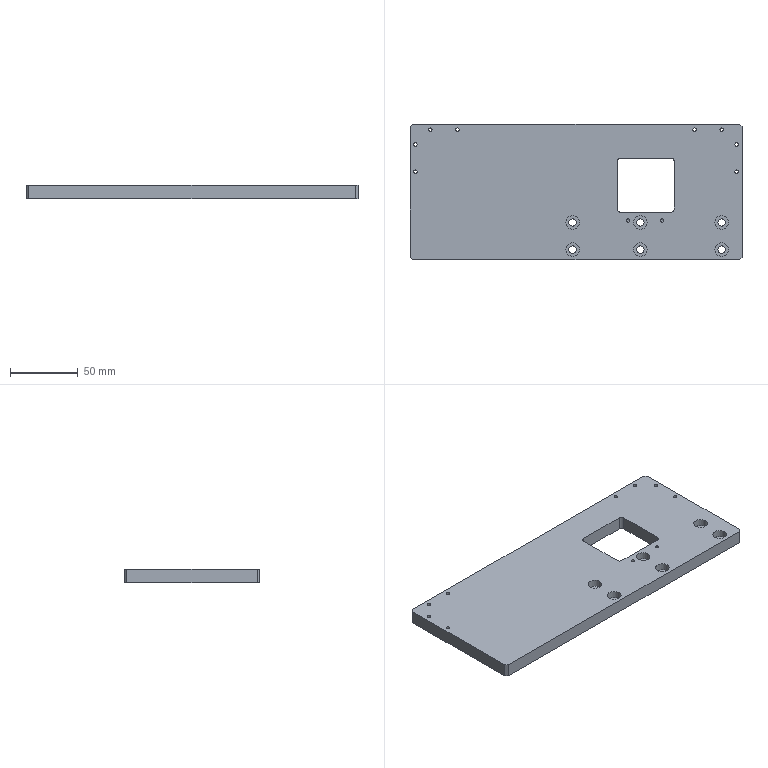Part | 1 solid | 48 faces | box 245 x 100 x 10 mm | volume 224502 mm3 | cylinder 26 | plane 20 | cone 2 | commonest cylinder face diameters 2.5 x10 5.5 x6 10 x6 4.871 x4
STEP:
#1=CARTESIAN_POINT('',(32.935,-15.,5.));
#2=VERTEX_POINT('',#1);
#3=CARTESIAN_POINT('',(70.065,-15.,5.));
#4=VERTEX_POINT('',#3);
#5=CARTESIAN_POINT('',(70.065,-15.,5.));
#6=DIRECTION('',(1.,0.,0.));
#7=VECTOR('',#6,1000.);
#8=LINE('',#5,#7);
#9=EDGE_CURVE('',#2,#4,#8,.T.);
#10=ORIENTED_EDGE('',*,*,#9,.T.);
#11=CARTESIAN_POINT('',(70.065,-15.,-5.));
#12=VERTEX_POINT('',#11);
#13=CARTESIAN_POINT('',(70.065,-15.,-5.));
#14=DIRECTION('',(0.,0.,1.));
#15=VECTOR('',#14,1000.);
#16=LINE('',#13,#15);
#17=EDGE_CURVE('',#12,#4,#16,.T.);
#18=ORIENTED_EDGE('',*,*,#17,.F.);
#19=CARTESIAN_POINT('',(32.935,-15.,-5.));
#20=VERTEX_POINT('',#19);
#21=CARTESIAN_POINT('',(70.065,-15.,-5.));
#22=DIRECTION('',(1.,0.,0.));
#23=VECTOR('',#22,1000.);
#24=LINE('',#21,#23);
#25=EDGE_CURVE('',#20,#12,#24,.T.);
#26=ORIENTED_EDGE('',*,*,#25,.F.);
#27=CARTESIAN_POINT('',(32.935,-15.,-5.));
#28=DIRECTION('',(0.,0.,1.));
#29=VECTOR('',#28,1000.);
#30=LINE('',#27,#29);
#31=EDGE_CURVE('',#20,#2,#30,.T.);
#32=ORIENTED_EDGE('',*,*,#31,.T.);
#33=EDGE_LOOP('',(#10,#18,#26,#32));
#34=FACE_BOUND('',#33,.T.);
#35=CARTESIAN_POINT('',(70.065,-15.,-5.));
#36=DIRECTION('',(0.,-1.,0.));
#37=DIRECTION('',(1.,0.,0.));
#38=AXIS2_PLACEMENT_3D('',#35,#36,#37);
#39=PLANE('',#38);
#40=ADVANCED_FACE('',(#34),#39,.F.);
#41=CARTESIAN_POINT('',(72.5,-12.565,5.));
#42=VERTEX_POINT('',#41);
#43=CARTESIAN_POINT('',(70.065,-12.565,5.));
#44=DIRECTION('',(0.,0.,1.));
#45=DIRECTION('',(1.,0.,0.));
#46=AXIS2_PLACEMENT_3D('',#43,#44,#45);
#47=CIRCLE('',#46,2.435);
#48=EDGE_CURVE('',#4,#42,#47,.T.);
#49=ORIENTED_EDGE('',*,*,#48,.T.);
#50=CARTESIAN_POINT('',(72.5,-12.565,-5.));
#51=VERTEX_POINT('',#50);
#52=CARTESIAN_POINT('',(72.5,-12.565,-5.));
#53=DIRECTION('',(0.,0.,1.));
#54=VECTOR('',#53,1000.);
#55=LINE('',#52,#54);
#56=EDGE_CURVE('',#51,#42,#55,.T.);
#57=ORIENTED_EDGE('',*,*,#56,.F.);
#58=CARTESIAN_POINT('',(70.065,-12.565,-5.));
#59=DIRECTION('',(0.,0.,1.));
#60=DIRECTION('',(1.,0.,0.));
#61=AXIS2_PLACEMENT_3D('',#58,#59,#60);
#62=CIRCLE('',#61,2.435);
#63=EDGE_CURVE('',#12,#51,#62,.T.);
#64=ORIENTED_EDGE('',*,*,#63,.F.);
#65=ORIENTED_EDGE('',*,*,#17,.T.);
#66=EDGE_LOOP('',(#49,#57,#64,#65));
#67=FACE_BOUND('',#66,.T.);
#68=CARTESIAN_POINT('',(70.065,-12.565,-5.));
#69=DIRECTION('',(0.,0.,1.));
#70=DIRECTION('',(1.,0.,0.));
#71=AXIS2_PLACEMENT_3D('',#68,#69,#70);
#72=CYLINDRICAL_SURFACE('',#71,2.435);
#73=ADVANCED_FACE('',(#67),#72,.F.);
#74=CARTESIAN_POINT('',(72.5,22.565,5.));
#75=VERTEX_POINT('',#74);
#76=CARTESIAN_POINT('',(72.5,-12.565,5.));
#77=DIRECTION('',(0.,1.,0.));
#78=VECTOR('',#77,1000.);
#79=LINE('',#76,#78);
#80=EDGE_CURVE('',#42,#75,#79,.T.);
#81=ORIENTED_EDGE('',*,*,#80,.T.);
#82=CARTESIAN_POINT('',(72.5,22.565,-5.));
#83=VERTEX_POINT('',#82);
#84=CARTESIAN_POINT('',(72.5,22.565,-5.));
#85=DIRECTION('',(0.,0.,1.));
#86=VECTOR('',#85,1000.);
#87=LINE('',#84,#86);
#88=EDGE_CURVE('',#83,#75,#87,.T.);
#89=ORIENTED_EDGE('',*,*,#88,.F.);
#90=CARTESIAN_POINT('',(72.5,-12.565,-5.));
#91=DIRECTION('',(0.,1.,0.));
#92=VECTOR('',#91,1000.);
#93=LINE('',#90,#92);
#94=EDGE_CURVE('',#51,#83,#93,.T.);
#95=ORIENTED_EDGE('',*,*,#94,.F.);
#96=ORIENTED_EDGE('',*,*,#56,.T.);
#97=EDGE_LOOP('',(#81,#89,#95,#96));
#98=FACE_BOUND('',#97,.T.);
#99=CARTESIAN_POINT('',(72.5,-12.565,-5.));
#100=DIRECTION('',(1.,0.,0.));
#101=DIRECTION('',(0.,0.,-1.));
#102=AXIS2_PLACEMENT_3D('',#99,#100,#101);
#103=PLANE('',#102);
#104=ADVANCED_FACE('',(#98),#103,.F.);
#105=CARTESIAN_POINT('',(70.065,25.,5.));
#106=VERTEX_POINT('',#105);
#107=CARTESIAN_POINT('',(70.065,22.565,5.));
#108=DIRECTION('',(0.,0.,1.));
#109=DIRECTION('',(1.,0.,0.));
#110=AXIS2_PLACEMENT_3D('',#107,#108,#109);
#111=CIRCLE('',#110,2.435);
#112=EDGE_CURVE('',#75,#106,#111,.T.);
#113=ORIENTED_EDGE('',*,*,#112,.T.);
#114=CARTESIAN_POINT('',(70.065,25.,-5.));
#115=VERTEX_POINT('',#114);
#116=CARTESIAN_POINT('',(70.065,25.,-5.));
#117=DIRECTION('',(0.,0.,1.));
#118=VECTOR('',#117,1000.);
#119=LINE('',#116,#118);
#120=EDGE_CURVE('',#115,#106,#119,.T.);
#121=ORIENTED_EDGE('',*,*,#120,.F.);
#122=CARTESIAN_POINT('',(70.065,22.565,-5.));
#123=DIRECTION('',(0.,0.,1.));
#124=DIRECTION('',(1.,0.,0.));
#125=AXIS2_PLACEMENT_3D('',#122,#123,#124);
#126=CIRCLE('',#125,2.435);
#127=EDGE_CURVE('',#83,#115,#126,.T.);
#128=ORIENTED_EDGE('',*,*,#127,.F.);
#129=ORIENTED_EDGE('',*,*,#88,.T.);
#130=EDGE_LOOP('',(#113,#121,#128,#129));
#131=FACE_BOUND('',#130,.T.);
#132=CARTESIAN_POINT('',(70.065,22.565,-5.));
#133=DIRECTION('',(0.,0.,1.));
#134=DIRECTION('',(1.,0.,0.));
#135=AXIS2_PLACEMENT_3D('',#132,#133,#134);
#136=CYLINDRICAL_SURFACE('',#135,2.435);
#137=ADVANCED_FACE('',(#131),#136,.F.);
#138=CARTESIAN_POINT('',(32.935,25.,5.));
#139=VERTEX_POINT('',#138);
#140=CARTESIAN_POINT('',(70.065,25.,5.));
#141=DIRECTION('',(-1.,0.,0.));
#142=VECTOR('',#141,1000.);
#143=LINE('',#140,#142);
#144=EDGE_CURVE('',#106,#139,#143,.T.);
#145=ORIENTED_EDGE('',*,*,#144,.T.);
#146=CARTESIAN_POINT('',(32.935,25.,-5.));
#147=VERTEX_POINT('',#146);
#148=CARTESIAN_POINT('',(32.935,25.,-5.));
#149=DIRECTION('',(0.,0.,1.));
#150=VECTOR('',#149,1000.);
#151=LINE('',#148,#150);
#152=EDGE_CURVE('',#147,#139,#151,.T.);
#153=ORIENTED_EDGE('',*,*,#152,.F.);
#154=CARTESIAN_POINT('',(70.065,25.,-5.));
#155=DIRECTION('',(-1.,0.,0.));
#156=VECTOR('',#155,1000.);
#157=LINE('',#154,#156);
#158=EDGE_CURVE('',#115,#147,#157,.T.);
#159=ORIENTED_EDGE('',*,*,#158,.F.);
#160=ORIENTED_EDGE('',*,*,#120,.T.);
#161=EDGE_LOOP('',(#145,#153,#159,#160));
#162=FACE_BOUND('',#161,.T.);
#163=CARTESIAN_POINT('',(70.065,25.,-5.));
#164=DIRECTION('',(0.,1.,0.));
#165=DIRECTION('',(-1.,0.,0.));
#166=AXIS2_PLACEMENT_3D('',#163,#164,#165);
#167=PLANE('',#166);
#168=ADVANCED_FACE('',(#162),#167,.F.);
#169=CARTESIAN_POINT('',(30.5,22.565,5.));
#170=VERTEX_POINT('',#169);
#171=CARTESIAN_POINT('',(32.935,22.565,5.));
#172=DIRECTION('',(0.,0.,1.));
#173=DIRECTION('',(1.,0.,0.));
#174=AXIS2_PLACEMENT_3D('',#171,#172,#173);
#175=CIRCLE('',#174,2.435);
#176=EDGE_CURVE('',#139,#170,#175,.T.);
#177=ORIENTED_EDGE('',*,*,#176,.T.);
#178=CARTESIAN_POINT('',(30.5,22.565,-5.));
#179=VERTEX_POINT('',#178);
#180=CARTESIAN_POINT('',(30.5,22.565,-5.));
#181=DIRECTION('',(0.,0.,1.));
#182=VECTOR('',#181,1000.);
#183=LINE('',#180,#182);
#184=EDGE_CURVE('',#179,#170,#183,.T.);
#185=ORIENTED_EDGE('',*,*,#184,.F.);
#186=CARTESIAN_POINT('',(32.935,22.565,-5.));
#187=DIRECTION('',(0.,0.,1.));
#188=DIRECTION('',(1.,0.,0.));
#189=AXIS2_PLACEMENT_3D('',#186,#187,#188);
#190=CIRCLE('',#189,2.435);
#191=EDGE_CURVE('',#147,#179,#190,.T.);
#192=ORIENTED_EDGE('',*,*,#191,.F.);
#193=ORIENTED_EDGE('',*,*,#152,.T.);
#194=EDGE_LOOP('',(#177,#185,#192,#193));
#195=FACE_BOUND('',#194,.T.);
#196=CARTESIAN_POINT('',(32.935,22.565,-5.));
#197=DIRECTION('',(0.,0.,1.));
#198=DIRECTION('',(1.,0.,0.));
#199=AXIS2_PLACEMENT_3D('',#196,#197,#198);
#200=CYLINDRICAL_SURFACE('',#199,2.435);
#201=ADVANCED_FACE('',(#195),#200,.F.);
#202=CARTESIAN_POINT('',(30.5,-12.565,5.));
#203=VERTEX_POINT('',#202);
#204=CARTESIAN_POINT('',(30.5,-12.565,5.));
#205=DIRECTION('',(0.,-1.,0.));
#206=VECTOR('',#205,1000.);
#207=LINE('',#204,#206);
#208=EDGE_CURVE('',#170,#203,#207,.T.);
#209=ORIENTED_EDGE('',*,*,#208,.T.);
#210=CARTESIAN_POINT('',(30.5,-12.565,-5.));
#211=VERTEX_POINT('',#210);
#212=CARTESIAN_POINT('',(30.5,-12.565,-5.));
#213=DIRECTION('',(0.,0.,1.));
#214=VECTOR('',#213,1000.);
#215=LINE('',#212,#214);
#216=EDGE_CURVE('',#211,#203,#215,.T.);
#217=ORIENTED_EDGE('',*,*,#216,.F.);
#218=CARTESIAN_POINT('',(30.5,-12.565,-5.));
#219=DIRECTION('',(0.,-1.,0.));
#220=VECTOR('',#219,1000.);
#221=LINE('',#218,#220);
#222=EDGE_CURVE('',#179,#211,#221,.T.);
#223=ORIENTED_EDGE('',*,*,#222,.F.);
#224=ORIENTED_EDGE('',*,*,#184,.T.);
#225=EDGE_LOOP('',(#209,#217,#223,#224));
#226=FACE_BOUND('',#225,.T.);
#227=CARTESIAN_POINT('',(30.5,-12.565,-5.));
#228=DIRECTION('',(-1.,0.,0.));
#229=DIRECTION('',(0.,0.,1.));
#230=AXIS2_PLACEMENT_3D('',#227,#228,#229);
#231=PLANE('',#230);
#232=ADVANCED_FACE('',(#226),#231,.F.);
#233=CARTESIAN_POINT('',(32.935,-12.565,5.));
#234=DIRECTION('',(0.,0.,1.));
#235=DIRECTION('',(-1.,0.,0.));
#236=AXIS2_PLACEMENT_3D('',#233,#234,#235);
#237=CIRCLE('',#236,2.435);
#238=EDGE_CURVE('',#203,#2,#237,.T.);
#239=ORIENTED_EDGE('',*,*,#238,.T.);
#240=ORIENTED_EDGE('',*,*,#31,.F.);
#241=CARTESIAN_POINT('',(32.935,-12.565,-5.));
#242=DIRECTION('',(0.,0.,1.));
#243=DIRECTION('',(-1.,0.,0.));
#244=AXIS2_PLACEMENT_3D('',#241,#242,#243);
#245=CIRCLE('',#244,2.435);
#246=EDGE_CURVE('',#211,#20,#245,.T.);
#247=ORIENTED_EDGE('',*,*,#246,.F.);
#248=ORIENTED_EDGE('',*,*,#216,.T.);
#249=EDGE_LOOP('',(#239,#240,#247,#248));
#250=FACE_BOUND('',#249,.T.);
#251=CARTESIAN_POINT('',(32.935,-12.565,-5.));
#252=DIRECTION('',(0.,0.,1.));
#253=DIRECTION('',(1.,0.,0.));
#254=AXIS2_PLACEMENT_3D('',#251,#252,#253);
#255=CYLINDRICAL_SURFACE('',#254,2.435);
#256=ADVANCED_FACE('',(#250),#255,.F.);
#257=CARTESIAN_POINT('',(-120.5,50.,5.));
#258=VERTEX_POINT('',#257);
#259=CARTESIAN_POINT('',(-122.5,48.,5.));
#260=VERTEX_POINT('',#259);
#261=CARTESIAN_POINT('',(-85.25,85.25,5.));
#262=DIRECTION('',(-0.7071,-0.7071,0.));
#263=VECTOR('',#262,1000.);
#264=LINE('',#261,#263);
#265=EDGE_CURVE('',#258,#260,#264,.T.);
#266=ORIENTED_EDGE('',*,*,#265,.F.);
#267=CARTESIAN_POINT('',(-120.5,50.,-5.));
#268=VERTEX_POINT('',#267);
#269=CARTESIAN_POINT('',(-120.5,50.,5.));
#270=DIRECTION('',(0.,0.,1.));
#271=VECTOR('',#270,1000.);
#272=LINE('',#269,#271);
#273=EDGE_CURVE('',#268,#258,#272,.T.);
#274=ORIENTED_EDGE('',*,*,#273,.F.);
#275=CARTESIAN_POINT('',(-122.5,48.,-5.));
#276=VERTEX_POINT('',#275);
#277=CARTESIAN_POINT('',(-122.5,48.,-5.));
#278=DIRECTION('',(0.7071,0.7071,0.));
#279=VECTOR('',#278,1000.);
#280=LINE('',#277,#279);
#281=EDGE_CURVE('',#276,#268,#280,.T.);
#282=ORIENTED_EDGE('',*,*,#281,.F.);
#283=CARTESIAN_POINT('',(-122.5,48.,5.));
#284=DIRECTION('',(0.,0.,-1.));
#285=VECTOR('',#284,1000.);
#286=LINE('',#283,#285);
#287=EDGE_CURVE('',#260,#276,#286,.T.);
#288=ORIENTED_EDGE('',*,*,#287,.F.);
#289=EDGE_LOOP('',(#266,#274,#282,#288));
#290=FACE_BOUND('',#289,.T.);
#291=CARTESIAN_POINT('',(-122.5,48.,5.));
#292=DIRECTION('',(0.7071,-0.7071,0.));
#293=DIRECTION('',(0.,0.,-1.));
#294=AXIS2_PLACEMENT_3D('',#291,#292,#293);
#295=PLANE('',#294);
#296=ADVANCED_FACE('',(#290),#295,.F.);
#297=CARTESIAN_POINT('',(-122.5,-48.,5.));
#298=VERTEX_POINT('',#297);
#299=CARTESIAN_POINT('',(-120.5,-50.,5.));
#300=VERTEX_POINT('',#299);
#301=CARTESIAN_POINT('',(-85.25,-85.25,5.));
#302=DIRECTION('',(0.7071,-0.7071,0.));
#303=VECTOR('',#302,1000.);
#304=LINE('',#301,#303);
#305=EDGE_CURVE('',#298,#300,#304,.T.);
#306=ORIENTED_EDGE('',*,*,#305,.F.);
#307=CARTESIAN_POINT('',(-122.5,-48.,-5.));
#308=VERTEX_POINT('',#307);
#309=CARTESIAN_POINT('',(-122.5,-48.,5.));
#310=DIRECTION('',(0.,0.,1.));
#311=VECTOR('',#310,1000.);
#312=LINE('',#309,#311);
#313=EDGE_CURVE('',#308,#298,#312,.T.);
#314=ORIENTED_EDGE('',*,*,#313,.F.);
#315=CARTESIAN_POINT('',(-120.5,-50.,-5.));
#316=VERTEX_POINT('',#315);
#317=CARTESIAN_POINT('',(-120.5,-50.,-5.));
#318=DIRECTION('',(-0.7071,0.7071,0.));
#319=VECTOR('',#318,1000.);
#320=LINE('',#317,#319);
#321=EDGE_CURVE('',#316,#308,#320,.T.);
#322=ORIENTED_EDGE('',*,*,#321,.F.);
#323=CARTESIAN_POINT('',(-120.5,-50.,5.));
#324=DIRECTION('',(0.,0.,-1.));
#325=VECTOR('',#324,1000.);
#326=LINE('',#323,#325);
#327=EDGE_CURVE('',#300,#316,#326,.T.);
#328=ORIENTED_EDGE('',*,*,#327,.F.);
#329=EDGE_LOOP('',(#306,#314,#322,#328));
#330=FACE_BOUND('',#329,.T.);
#331=CARTESIAN_POINT('',(-120.5,-50.,5.));
#332=DIRECTION('',(0.7071,0.7071,0.));
#333=DIRECTION('',(0.,0.,-1.));
#334=AXIS2_PLACEMENT_3D('',#331,#332,#333);
#335=PLANE('',#334);
#336=ADVANCED_FACE('',(#330),#335,.F.);
#337=CARTESIAN_POINT('',(120.5,-50.,5.));
#338=VERTEX_POINT('',#337);
#339=CARTESIAN_POINT('',(122.5,-48.,5.));
#340=VERTEX_POINT('',#339);
#341=CARTESIAN_POINT('',(85.25,-85.25,5.));
#342=DIRECTION('',(0.7071,0.7071,0.));
#343=VECTOR('',#342,1000.);
#344=LINE('',#341,#343);
#345=EDGE_CURVE('',#338,#340,#344,.T.);
#346=ORIENTED_EDGE('',*,*,#345,.F.);
#347=CARTESIAN_POINT('',(120.5,-50.,-5.));
#348=VERTEX_POINT('',#347);
#349=CARTESIAN_POINT('',(120.5,-50.,5.));
#350=DIRECTION('',(0.,0.,1.));
#351=VECTOR('',#350,1000.);
#352=LINE('',#349,#351);
#353=EDGE_CURVE('',#348,#338,#352,.T.);
#354=ORIENTED_EDGE('',*,*,#353,.F.);
#355=CARTESIAN_POINT('',(122.5,-48.,-5.));
#356=VERTEX_POINT('',#355);
#357=CARTESIAN_POINT('',(122.5,-48.,-5.));
#358=DIRECTION('',(-0.7071,-0.7071,0.));
#359=VECTOR('',#358,1000.);
#360=LINE('',#357,#359);
#361=EDGE_CURVE('',#356,#348,#360,.T.);
#362=ORIENTED_EDGE('',*,*,#361,.F.);
#363=CARTESIAN_POINT('',(122.5,-48.,5.));
#364=DIRECTION('',(0.,0.,-1.));
#365=VECTOR('',#364,1000.);
#366=LINE('',#363,#365);
#367=EDGE_CURVE('',#340,#356,#366,.T.);
#368=ORIENTED_EDGE('',*,*,#367,.F.);
#369=EDGE_LOOP('',(#346,#354,#362,#368));
#370=FACE_BOUND('',#369,.T.);
#371=CARTESIAN_POINT('',(122.5,-48.,5.));
#372=DIRECTION('',(-0.7071,0.7071,0.));
#373=DIRECTION('',(0.,0.,-1.));
#374=AXIS2_PLACEMENT_3D('',#371,#372,#373);
#375=PLANE('',#374);
#376=ADVANCED_FACE('',(#370),#375,.F.);
#377=CARTESIAN_POINT('',(122.5,48.,5.));
#378=VERTEX_POINT('',#377);
#379=CARTESIAN_POINT('',(120.5,50.,5.));
#380=VERTEX_POINT('',#379);
#381=CARTESIAN_POINT('',(85.25,85.25,5.));
#382=DIRECTION('',(-0.7071,0.7071,0.));
#383=VECTOR('',#382,1000.);
#384=LINE('',#381,#383);
#385=EDGE_CURVE('',#378,#380,#384,.T.);
#386=ORIENTED_EDGE('',*,*,#385,.F.);
#387=CARTESIAN_POINT('',(122.5,48.,-5.));
#388=VERTEX_POINT('',#387);
#389=CARTESIAN_POINT('',(122.5,48.,5.));
#390=DIRECTION('',(0.,0.,1.));
#391=VECTOR('',#390,1000.);
#392=LINE('',#389,#391);
#393=EDGE_CURVE('',#388,#378,#392,.T.);
#394=ORIENTED_EDGE('',*,*,#393,.F.);
#395=CARTESIAN_POINT('',(120.5,50.,-5.));
#396=VERTEX_POINT('',#395);
#397=CARTESIAN_POINT('',(120.5,50.,-5.));
#398=DIRECTION('',(0.7071,-0.7071,0.));
#399=VECTOR('',#398,1000.);
#400=LINE('',#397,#399);
#401=EDGE_CURVE('',#396,#388,#400,.T.);
#402=ORIENTED_EDGE('',*,*,#401,.F.);
#403=CARTESIAN_POINT('',(120.5,50.,5.));
#404=DIRECTION('',(0.,0.,-1.));
#405=VECTOR('',#404,1000.);
#406=LINE('',#403,#405);
#407=EDGE_CURVE('',#380,#396,#406,.T.);
#408=ORIENTED_EDGE('',*,*,#407,.F.);
#409=EDGE_LOOP('',(#386,#394,#402,#408));
#410=FACE_BOUND('',#409,.T.);
#411=CARTESIAN_POINT('',(120.5,50.,5.));
#412=DIRECTION('',(-0.7071,-0.7071,0.));
#413=DIRECTION('',(0.,0.,-1.));
#414=AXIS2_PLACEMENT_3D('',#411,#412,#413);
#415=PLANE('',#414);
#416=ADVANCED_FACE('',(#410),#415,.F.);
#417=CARTESIAN_POINT('',(2.5,-42.5,-0.4));
#418=VERTEX_POINT('',#417);
#419=CARTESIAN_POINT('',(-2.5,-42.5,-0.4));
#420=DIRECTION('',(0.,0.,1.));
#421=DIRECTION('',(1.,0.,0.));
#422=AXIS2_PLACEMENT_3D('',#419,#420,#421);
#423=CIRCLE('',#422,5.);
#424=EDGE_CURVE('',#418,#418,#423,.T.);
#425=ORIENTED_EDGE('',*,*,#424,.T.);
#426=EDGE_LOOP('',(#425));
#427=FACE_BOUND('',#426,.T.);
#428=CARTESIAN_POINT('',(0.25,-42.5,-0.4));
#429=VERTEX_POINT('',#428);
#430=CARTESIAN_POINT('',(-2.5,-42.5,-0.4));
#431=DIRECTION('',(0.,0.,1.));
#432=DIRECTION('',(1.,0.,0.));
#433=AXIS2_PLACEMENT_3D('',#430,#431,#432);
#434=CIRCLE('',#433,2.75);
#435=EDGE_CURVE('',#429,#429,#434,.T.);
#436=ORIENTED_EDGE('',*,*,#435,.F.);
#437=EDGE_LOOP('',(#436));
#438=FACE_BOUND('',#437,.T.);
#439=CARTESIAN_POINT('',(0.25,-42.5,-0.4));
#440=DIRECTION('',(0.,0.,-1.));
#441=DIRECTION('',(-1.,0.,0.));
#442=AXIS2_PLACEMENT_3D('',#439,#440,#441);
#443=PLANE('',#442);
#444=ADVANCED_FACE('',(#427,#438),#443,.F.);
#445=CARTESIAN_POINT('',(42.5,-42.5,-0.4));
#446=VERTEX_POINT('',#445);
#447=CARTESIAN_POINT('',(47.5,-42.5,-0.4));
#448=DIRECTION('',(0.,0.,1.));
#449=DIRECTION('',(-1.,0.,0.));
#450=AXIS2_PLACEMENT_3D('',#447,#448,#449);
#451=CIRCLE('',#450,5.);
#452=EDGE_CURVE('',#446,#446,#451,.T.);
#453=ORIENTED_EDGE('',*,*,#452,.T.);
#454=EDGE_LOOP('',(#453));
#455=FACE_BOUND('',#454,.T.);
#456=CARTESIAN_POINT('',(44.75,-42.5,-0.4));
#457=VERTEX_POINT('',#456);
#458=CARTESIAN_POINT('',(47.5,-42.5,-0.4));
#459=DIRECTION('',(0.,0.,1.));
#460=DIRECTION('',(-1.,0.,0.));
#461=AXIS2_PLACEMENT_3D('',#458,#459,#460);
#462=CIRCLE('',#461,2.75);
#463=EDGE_CURVE('',#457,#457,#462,.T.);
#464=ORIENTED_EDGE('',*,*,#463,.F.);
#465=EDGE_LOOP('',(#464));
#466=FACE_BOUND('',#465,.T.);
#467=CARTESIAN_POINT('',(0.25,-42.5,-0.4));
#468=DIRECTION('',(0.,0.,-1.));
#469=DIRECTION('',(-1.,0.,0.));
#470=AXIS2_PLACEMENT_3D('',#467,#468,#469);
#471=PLANE('',#470);
#472=ADVANCED_FACE('',(#455,#466),#471,.F.);
#473=CARTESIAN_POINT('',(102.5,-42.5,-0.4));
#474=VERTEX_POINT('',#473);
#475=CARTESIAN_POINT('',(107.5,-42.5,-0.4));
#476=DIRECTION('',(0.,0.,1.));
#477=DIRECTION('',(-1.,0.,0.));
#478=AXIS2_PLACEMENT_3D('',#475,#476,#477);
#479=CIRCLE('',#478,5.);
#480=EDGE_CURVE('',#474,#474,#479,.T.);
#481=ORIENTED_EDGE('',*,*,#480,.T.);
#482=EDGE_LOOP('',(#481));
#483=FACE_BOUND('',#482,.T.);
#484=CARTESIAN_POINT('',(104.75,-42.5,-0.4));
#485=VERTEX_POINT('',#484);
#486=CARTESIAN_POINT('',(107.5,-42.5,-0.4));
#487=DIRECTION('',(0.,0.,1.));
#488=DIRECTION('',(-1.,0.,0.));
#489=AXIS2_PLACEMENT_3D('',#486,#487,#488);
#490=CIRCLE('',#489,2.75);
#491=EDGE_CURVE('',#485,#485,#490,.T.);
#492=ORIENTED_EDGE('',*,*,#491,.F.);
#493=EDGE_LOOP('',(#492));
#494=FACE_BOUND('',#493,.T.);
#495=CARTESIAN_POINT('',(0.25,-42.5,-0.4));
#496=DIRECTION('',(0.,0.,-1.));
#497=DIRECTION('',(-1.,0.,0.));
#498=AXIS2_PLACEMENT_3D('',#495,#496,#497);
#499=PLANE('',#498);
#500=ADVANCED_FACE('',(#483,#494),#499,.F.);
#501=CARTESIAN_POINT('',(-7.5,-22.5,-0.4));
#502=VERTEX_POINT('',#501);
#503=CARTESIAN_POINT('',(-2.5,-22.5,-0.4));
#504=DIRECTION('',(0.,0.,1.));
#505=DIRECTION('',(-1.,0.,0.));
#506=AXIS2_PLACEMENT_3D('',#503,#504,#505);
#507=CIRCLE('',#506,5.);
#508=EDGE_CURVE('',#502,#502,#507,.T.);
#509=ORIENTED_EDGE('',*,*,#508,.T.);
#510=EDGE_LOOP('',(#509));
#511=FACE_BOUND('',#510,.T.);
#512=CARTESIAN_POINT('',(-5.25,-22.5,-0.4));
#513=VERTEX_POINT('',#512);
#514=CARTESIAN_POINT('',(-2.5,-22.5,-0.4));
#515=DIRECTION('',(0.,0.,1.));
#516=DIRECTION('',(-1.,0.,0.));
#517=AXIS2_PLACEMENT_3D('',#514,#515,#516);
#518=CIRCLE('',#517,2.75);
#519=EDGE_CURVE('',#513,#513,#518,.T.);
#520=ORIENTED_EDGE('',*,*,#519,.F.);
#521=EDGE_LOOP('',(#520));
#522=FACE_BOUND('',#521,.T.);
#523=CARTESIAN_POINT('',(0.25,-42.5,-0.4));
#524=DIRECTION('',(0.,0.,-1.));
#525=DIRECTION('',(-1.,0.,0.));
#526=AXIS2_PLACEMENT_3D('',#523,#524,#525);
#527=PLANE('',#526);
#528=ADVANCED_FACE('',(#511,#522),#527,.F.);
#529=CARTESIAN_POINT('',(42.5,-22.5,-0.4));
#530=VERTEX_POINT('',#529);
#531=CARTESIAN_POINT('',(47.5,-22.5,-0.4));
#532=DIRECTION('',(0.,0.,1.));
#533=DIRECTION('',(-1.,0.,0.));
#534=AXIS2_PLACEMENT_3D('',#531,#532,#533);
#535=CIRCLE('',#534,5.);
#536=EDGE_CURVE('',#530,#530,#535,.T.);
#537=ORIENTED_EDGE('',*,*,#536,.T.);
#538=EDGE_LOOP('',(#537));
#539=FACE_BOUND('',#538,.T.);
#540=CARTESIAN_POINT('',(44.75,-22.5,-0.4));
#541=VERTEX_POINT('',#540);
#542=CARTESIAN_POINT('',(47.5,-22.5,-0.4));
#543=DIRECTION('',(0.,0.,1.));
#544=DIRECTION('',(-1.,0.,0.));
#545=AXIS2_PLACEMENT_3D('',#542,#543,#544);
#546=CIRCLE('',#545,2.75);
#547=EDGE_CURVE('',#541,#541,#546,.T.);
#548=ORIENTED_EDGE('',*,*,#547,.F.);
#549=EDGE_LOOP('',(#548));
#550=FACE_BOUND('',#549,.T.);
#551=CARTESIAN_POINT('',(0.25,-42.5,-0.4));
#552=DIRECTION('',(0.,0.,-1.));
#553=DIRECTION('',(-1.,0.,0.));
#554=AXIS2_PLACEMENT_3D('',#551,#552,#553);
#555=PLANE('',#554);
#556=ADVANCED_FACE('',(#539,#550),#555,.F.);
#557=CARTESIAN_POINT('',(102.5,-22.5,-0.4));
#558=VERTEX_POINT('',#557);
#559=CARTESIAN_POINT('',(107.5,-22.5,-0.4));
#560=DIRECTION('',(0.,0.,1.));
#561=DIRECTION('',(-1.,0.,0.));
#562=AXIS2_PLACEMENT_3D('',#559,#560,#561);
#563=CIRCLE('',#562,5.);
#564=EDGE_CURVE('',#558,#558,#563,.T.);
#565=ORIENTED_EDGE('',*,*,#564,.T.);
#566=EDGE_LOOP('',(#565));
#567=FACE_BOUND('',#566,.T.);
#568=CARTESIAN_POINT('',(104.75,-22.5,-0.4));
#569=VERTEX_POINT('',#568);
#570=CARTESIAN_POINT('',(107.5,-22.5,-0.4));
#571=DIRECTION('',(0.,0.,1.));
#572=DIRECTION('',(-1.,0.,0.));
#573=AXIS2_PLACEMENT_3D('',#570,#571,#572);
#574=CIRCLE('',#573,2.75);
#575=EDGE_CURVE('',#569,#569,#574,.T.);
#576=ORIENTED_EDGE('',*,*,#575,.F.);
#577=EDGE_LOOP('',(#576));
#578=FACE_BOUND('',#577,.T.);
#579=CARTESIAN_POINT('',(0.25,-42.5,-0.4));
#580=DIRECTION('',(0.,0.,-1.));
#581=DIRECTION('',(-1.,0.,0.));
#582=AXIS2_PLACEMENT_3D('',#579,#580,#581);
#583=PLANE('',#582);
#584=ADVANCED_FACE('',(#567,#578),#583,.F.);
#585=CARTESIAN_POINT('',(-122.5,50.,-5.));
#586=DIRECTION('',(-1.,0.,0.));
#587=VECTOR('',#586,1000.);
#588=LINE('',#585,#587);
#589=EDGE_CURVE('',#396,#268,#588,.T.);
#590=ORIENTED_EDGE('',*,*,#589,.F.);
#591=ORIENTED_EDGE('',*,*,#401,.T.);
#592=CARTESIAN_POINT('',(122.5,50.,-5.));
#593=DIRECTION('',(0.,1.,0.));
#594=VECTOR('',#593,1000.);
#595=LINE('',#592,#594);
#596=EDGE_CURVE('',#356,#388,#595,.T.);
#597=ORIENTED_EDGE('',*,*,#596,.F.);
#598=ORIENTED_EDGE('',*,*,#361,.T.);
#599=CARTESIAN_POINT('',(-122.5,-50.,-5.));
#600=DIRECTION('',(1.,0.,0.));
#601=VECTOR('',#600,1000.);
#602=LINE('',#599,#601);
#603=EDGE_CURVE('',#316,#348,#602,.T.);
#604=ORIENTED_EDGE('',*,*,#603,.F.);
#605=ORIENTED_EDGE('',*,*,#321,.T.);
#606=CARTESIAN_POINT('',(-122.5,50.,-5.));
#607=DIRECTION('',(0.,-1.,0.));
#608=VECTOR('',#607,1000.);
#609=LINE('',#606,#608);
#610=EDGE_CURVE('',#276,#308,#609,.T.);
#611=ORIENTED_EDGE('',*,*,#610,.F.);
#612=ORIENTED_EDGE('',*,*,#281,.T.);
#613=EDGE_LOOP('',(#590,#591,#597,#598,#604,#605,#611,#612));
#614=FACE_BOUND('',#613,.T.);
#615=CARTESIAN_POINT('',(110.25,-22.5,-5.));
#616=VERTEX_POINT('',#615);
#617=CARTESIAN_POINT('',(107.5,-22.5,-5.));
#618=DIRECTION('',(0.,0.,1.));
#619=DIRECTION('',(1.,0.,0.));
#620=AXIS2_PLACEMENT_3D('',#617,#618,#619);
#621=CIRCLE('',#620,2.75);
#622=EDGE_CURVE('',#616,#616,#621,.T.);
#623=ORIENTED_EDGE('',*,*,#622,.T.);
#624=EDGE_LOOP('',(#623));
#625=FACE_BOUND('',#624,.T.);
#626=CARTESIAN_POINT('',(50.25,-22.5,-5.));
#627=VERTEX_POINT('',#626);
#628=CARTESIAN_POINT('',(47.5,-22.5,-5.));
#629=DIRECTION('',(0.,0.,1.));
#630=DIRECTION('',(1.,0.,0.));
#631=AXIS2_PLACEMENT_3D('',#628,#629,#630);
#632=CIRCLE('',#631,2.75);
#633=EDGE_CURVE('',#627,#627,#632,.T.);
#634=ORIENTED_EDGE('',*,*,#633,.T.);
#635=EDGE_LOOP('',(#634));
#636=FACE_BOUND('',#635,.T.);
#637=CARTESIAN_POINT('',(0.25,-22.5,-5.));
#638=VERTEX_POINT('',#637);
#639=CARTESIAN_POINT('',(-2.5,-22.5,-5.));
#640=DIRECTION('',(0.,0.,1.));
#641=DIRECTION('',(1.,0.,0.));
#642=AXIS2_PLACEMENT_3D('',#639,#640,#641);
#643=CIRCLE('',#642,2.75);
#644=EDGE_CURVE('',#638,#638,#643,.T.);
#645=ORIENTED_EDGE('',*,*,#644,.T.);
#646=EDGE_LOOP('',(#645));
#647=FACE_BOUND('',#646,.T.);
#648=CARTESIAN_POINT('',(110.25,-42.5,-5.));
#649=VERTEX_POINT('',#648);
#650=CARTESIAN_POINT('',(107.5,-42.5,-5.));
#651=DIRECTION('',(0.,0.,1.));
#652=DIRECTION('',(1.,0.,0.));
#653=AXIS2_PLACEMENT_3D('',#650,#651,#652);
#654=CIRCLE('',#653,2.75);
#655=EDGE_CURVE('',#649,#649,#654,.T.);
#656=ORIENTED_EDGE('',*,*,#655,.T.);
#657=EDGE_LOOP('',(#656));
#658=FACE_BOUND('',#657,.T.);
#659=CARTESIAN_POINT('',(50.25,-42.5,-5.));
#660=VERTEX_POINT('',#659);
#661=CARTESIAN_POINT('',(47.5,-42.5,-5.));
#662=DIRECTION('',(0.,0.,1.));
#663=DIRECTION('',(1.,0.,0.));
#664=AXIS2_PLACEMENT_3D('',#661,#662,#663);
#665=CIRCLE('',#664,2.75);
#666=EDGE_CURVE('',#660,#660,#665,.T.);
#667=ORIENTED_EDGE('',*,*,#666,.T.);
#668=EDGE_LOOP('',(#667));
#669=FACE_BOUND('',#668,.T.);
#670=CARTESIAN_POINT('',(0.25,-42.5,-5.));
#671=VERTEX_POINT('',#670);
#672=CARTESIAN_POINT('',(-2.5,-42.5,-5.));
#673=DIRECTION('',(0.,0.,1.));
#674=DIRECTION('',(1.,0.,0.));
#675=AXIS2_PLACEMENT_3D('',#672,#673,#674);
#676=CIRCLE('',#675,2.75);
#677=EDGE_CURVE('',#671,#671,#676,.T.);
#678=ORIENTED_EDGE('',*,*,#677,.T.);
#679=EDGE_LOOP('',(#678));
#680=FACE_BOUND('',#679,.T.);
#681=CARTESIAN_POINT('',(119.75,15.,-5.));
#682=VERTEX_POINT('',#681);
#683=CARTESIAN_POINT('',(118.5,15.,-5.));
#684=DIRECTION('',(0.,0.,1.));
#685=DIRECTION('',(1.,0.,0.));
#686=AXIS2_PLACEMENT_3D('',#683,#684,#685);
#687=CIRCLE('',#686,1.25);
#688=EDGE_CURVE('',#682,#682,#687,.T.);
#689=ORIENTED_EDGE('',*,*,#688,.T.);
#690=EDGE_LOOP('',(#689));
#691=FACE_BOUND('',#690,.T.);
#692=CARTESIAN_POINT('',(119.75,35.,-5.));
#693=VERTEX_POINT('',#692);
#694=CARTESIAN_POINT('',(118.5,35.,-5.));
#695=DIRECTION('',(0.,0.,1.));
#696=DIRECTION('',(1.,0.,0.));
#697=AXIS2_PLACEMENT_3D('',#694,#695,#696);
#698=CIRCLE('',#697,1.25);
#699=EDGE_CURVE('',#693,#693,#698,.T.);
#700=ORIENTED_EDGE('',*,*,#699,.T.);
#701=EDGE_LOOP('',(#700));
#702=FACE_BOUND('',#701,.T.);
#703=CARTESIAN_POINT('',(108.75,46.,-5.));
#704=VERTEX_POINT('',#703);
#705=CARTESIAN_POINT('',(107.5,46.,-5.));
#706=DIRECTION('',(0.,0.,1.));
#707=DIRECTION('',(1.,0.,0.));
#708=AXIS2_PLACEMENT_3D('',#705,#706,#707);
#709=CIRCLE('',#708,1.25);
#710=EDGE_CURVE('',#704,#704,#709,.T.);
#711=ORIENTED_EDGE('',*,*,#710,.T.);
#712=EDGE_LOOP('',(#711));
#713=FACE_BOUND('',#712,.T.);
#714=CARTESIAN_POINT('',(88.75,46.,-5.));
#715=VERTEX_POINT('',#714);
#716=CARTESIAN_POINT('',(87.5,46.,-5.));
#717=DIRECTION('',(0.,0.,1.));
#718=DIRECTION('',(1.,0.,0.));
#719=AXIS2_PLACEMENT_3D('',#716,#717,#718);
#720=CIRCLE('',#719,1.25);
#721=EDGE_CURVE('',#715,#715,#720,.T.);
#722=ORIENTED_EDGE('',*,*,#721,.T.);
#723=EDGE_LOOP('',(#722));
#724=FACE_BOUND('',#723,.T.);
#725=CARTESIAN_POINT('',(-86.25,46.,-5.));
#726=VERTEX_POINT('',#725);
#727=CARTESIAN_POINT('',(-87.5,46.,-5.));
#728=DIRECTION('',(0.,0.,1.));
#729=DIRECTION('',(1.,0.,0.));
#730=AXIS2_PLACEMENT_3D('',#727,#728,#729);
#731=CIRCLE('',#730,1.25);
#732=EDGE_CURVE('',#726,#726,#731,.T.);
#733=ORIENTED_EDGE('',*,*,#732,.T.);
#734=EDGE_LOOP('',(#733));
#735=FACE_BOUND('',#734,.T.);
#736=CARTESIAN_POINT('',(-106.25,46.,-5.));
#737=VERTEX_POINT('',#736);
#738=CARTESIAN_POINT('',(-107.5,46.,-5.));
#739=DIRECTION('',(0.,0.,1.));
#740=DIRECTION('',(1.,0.,0.));
#741=AXIS2_PLACEMENT_3D('',#738,#739,#740);
#742=CIRCLE('',#741,1.25);
#743=EDGE_CURVE('',#737,#737,#742,.T.);
#744=ORIENTED_EDGE('',*,*,#743,.T.);
#745=EDGE_LOOP('',(#744));
#746=FACE_BOUND('',#745,.T.);
#747=CARTESIAN_POINT('',(-117.25,35.,-5.));
#748=VERTEX_POINT('',#747);
#749=CARTESIAN_POINT('',(-118.5,35.,-5.));
#750=DIRECTION('',(0.,0.,1.));
#751=DIRECTION('',(1.,0.,0.));
#752=AXIS2_PLACEMENT_3D('',#749,#750,#751);
#753=CIRCLE('',#752,1.25);
#754=EDGE_CURVE('',#748,#748,#753,.T.);
#755=ORIENTED_EDGE('',*,*,#754,.T.);
#756=EDGE_LOOP('',(#755));
#757=FACE_BOUND('',#756,.T.);
#758=CARTESIAN_POINT('',(-117.25,15.,-5.));
#759=VERTEX_POINT('',#758);
#760=CARTESIAN_POINT('',(-118.5,15.,-5.));
#761=DIRECTION('',(0.,0.,1.));
#762=DIRECTION('',(1.,0.,0.));
#763=AXIS2_PLACEMENT_3D('',#760,#761,#762);
#764=CIRCLE('',#763,1.25);
#765=EDGE_CURVE('',#759,#759,#764,.T.);
#766=ORIENTED_EDGE('',*,*,#765,.T.);
#767=EDGE_LOOP('',(#766));
#768=FACE_BOUND('',#767,.T.);
#769=ORIENTED_EDGE('',*,*,#222,.T.);
#770=ORIENTED_EDGE('',*,*,#246,.T.);
#771=ORIENTED_EDGE('',*,*,#25,.T.);
#772=ORIENTED_EDGE('',*,*,#63,.T.);
#773=ORIENTED_EDGE('',*,*,#94,.T.);
#774=ORIENTED_EDGE('',*,*,#127,.T.);
#775=ORIENTED_EDGE('',*,*,#158,.T.);
#776=ORIENTED_EDGE('',*,*,#191,.T.);
#777=EDGE_LOOP('',(#769,#770,#771,#772,#773,#774,#775,#776));
#778=FACE_BOUND('',#777,.T.);
#779=CARTESIAN_POINT('',(0.,0.,-5.));
#780=DIRECTION('',(0.,0.,1.));
#781=DIRECTION('',(1.,0.,0.));
#782=AXIS2_PLACEMENT_3D('',#779,#780,#781);
#783=PLANE('',#782);
#784=ADVANCED_FACE('',(#614,#625,#636,#647,#658,#669,#680,#691,#702,#713,#724,#735,#746,#757,#768,#778),#783,.F.);
#785=CARTESIAN_POINT('',(122.5,50.,5.));
#786=DIRECTION('',(0.,1.,0.));
#787=VECTOR('',#786,1000.);
#788=LINE('',#785,#787);
#789=EDGE_CURVE('',#340,#378,#788,.T.);
#790=ORIENTED_EDGE('',*,*,#789,.T.);
#791=ORIENTED_EDGE('',*,*,#385,.T.);
#792=CARTESIAN_POINT('',(-122.5,50.,5.));
#793=DIRECTION('',(-1.,0.,0.));
#794=VECTOR('',#793,1000.);
#795=LINE('',#792,#794);
#796=EDGE_CURVE('',#380,#258,#795,.T.);
#797=ORIENTED_EDGE('',*,*,#796,.T.);
#798=ORIENTED_EDGE('',*,*,#265,.T.);
#799=CARTESIAN_POINT('',(-122.5,50.,5.));
#800=DIRECTION('',(0.,-1.,0.));
#801=VECTOR('',#800,1000.);
#802=LINE('',#799,#801);
#803=EDGE_CURVE('',#260,#298,#802,.T.);
#804=ORIENTED_EDGE('',*,*,#803,.T.);
#805=ORIENTED_EDGE('',*,*,#305,.T.);
#806=CARTESIAN_POINT('',(-122.5,-50.,5.));
#807=DIRECTION('',(1.,0.,0.));
#808=VECTOR('',#807,1000.);
#809=LINE('',#806,#808);
#810=EDGE_CURVE('',#300,#338,#809,.T.);
#811=ORIENTED_EDGE('',*,*,#810,.T.);
#812=ORIENTED_EDGE('',*,*,#345,.T.);
#813=EDGE_LOOP('',(#790,#791,#797,#798,#804,#805,#811,#812));
#814=FACE_BOUND('',#813,.T.);
#815=CARTESIAN_POINT('',(112.5,-22.5,5.));
#816=VERTEX_POINT('',#815);
#817=CARTESIAN_POINT('',(107.5,-22.5,5.));
#818=DIRECTION('',(0.,0.,1.));
#819=DIRECTION('',(1.,0.,0.));
#820=AXIS2_PLACEMENT_3D('',#817,#818,#819);
#821=CIRCLE('',#820,5.);
#822=EDGE_CURVE('',#816,#816,#821,.T.);
#823=ORIENTED_EDGE('',*,*,#822,.F.);
#824=EDGE_LOOP('',(#823));
#825=FACE_BOUND('',#824,.T.);
#826=CARTESIAN_POINT('',(52.5,-22.5,5.));
#827=VERTEX_POINT('',#826);
#828=CARTESIAN_POINT('',(47.5,-22.5,5.));
#829=DIRECTION('',(0.,0.,1.));
#830=DIRECTION('',(1.,0.,0.));
#831=AXIS2_PLACEMENT_3D('',#828,#829,#830);
#832=CIRCLE('',#831,5.);
#833=EDGE_CURVE('',#827,#827,#832,.T.);
#834=ORIENTED_EDGE('',*,*,#833,.F.);
#835=EDGE_LOOP('',(#834));
#836=FACE_BOUND('',#835,.T.);
#837=CARTESIAN_POINT('',(2.5,-22.5,5.));
#838=VERTEX_POINT('',#837);
#839=CARTESIAN_POINT('',(-2.5,-22.5,5.));
#840=DIRECTION('',(0.,0.,1.));
#841=DIRECTION('',(1.,0.,0.));
#842=AXIS2_PLACEMENT_3D('',#839,#840,#841);
#843=CIRCLE('',#842,5.);
#844=EDGE_CURVE('',#838,#838,#843,.T.);
#845=ORIENTED_EDGE('',*,*,#844,.F.);
#846=EDGE_LOOP('',(#845));
#847=FACE_BOUND('',#846,.T.);
#848=CARTESIAN_POINT('',(112.5,-42.5,5.));
#849=VERTEX_POINT('',#848);
#850=CARTESIAN_POINT('',(107.5,-42.5,5.));
#851=DIRECTION('',(0.,0.,1.));
#852=DIRECTION('',(1.,0.,0.));
#853=AXIS2_PLACEMENT_3D('',#850,#851,#852);
#854=CIRCLE('',#853,5.);
#855=EDGE_CURVE('',#849,#849,#854,.T.);
#856=ORIENTED_EDGE('',*,*,#855,.F.);
#857=EDGE_LOOP('',(#856));
#858=FACE_BOUND('',#857,.T.);
#859=CARTESIAN_POINT('',(52.5,-42.5,5.));
#860=VERTEX_POINT('',#859);
#861=CARTESIAN_POINT('',(47.5,-42.5,5.));
#862=DIRECTION('',(0.,0.,1.));
#863=DIRECTION('',(1.,0.,0.));
#864=AXIS2_PLACEMENT_3D('',#861,#862,#863);
#865=CIRCLE('',#864,5.);
#866=EDGE_CURVE('',#860,#860,#865,.T.);
#867=ORIENTED_EDGE('',*,*,#866,.F.);
#868=EDGE_LOOP('',(#867));
#869=FACE_BOUND('',#868,.T.);
#870=CARTESIAN_POINT('',(2.5,-42.5,5.));
#871=VERTEX_POINT('',#870);
#872=CARTESIAN_POINT('',(-2.5,-42.5,5.));
#873=DIRECTION('',(0.,0.,1.));
#874=DIRECTION('',(1.,0.,0.));
#875=AXIS2_PLACEMENT_3D('',#872,#873,#874);
#876=CIRCLE('',#875,5.);
#877=EDGE_CURVE('',#871,#871,#876,.T.);
#878=ORIENTED_EDGE('',*,*,#877,.F.);
#879=EDGE_LOOP('',(#878));
#880=FACE_BOUND('',#879,.T.);
#881=CARTESIAN_POINT('',(119.75,15.,5.));
#882=VERTEX_POINT('',#881);
#883=CARTESIAN_POINT('',(118.5,15.,5.));
#884=DIRECTION('',(0.,0.,1.));
#885=DIRECTION('',(1.,0.,0.));
#886=AXIS2_PLACEMENT_3D('',#883,#884,#885);
#887=CIRCLE('',#886,1.25);
#888=EDGE_CURVE('',#882,#882,#887,.T.);
#889=ORIENTED_EDGE('',*,*,#888,.F.);
#890=EDGE_LOOP('',(#889));
#891=FACE_BOUND('',#890,.T.);
#892=CARTESIAN_POINT('',(119.75,35.,5.));
#893=VERTEX_POINT('',#892);
#894=CARTESIAN_POINT('',(118.5,35.,5.));
#895=DIRECTION('',(0.,0.,1.));
#896=DIRECTION('',(1.,0.,0.));
#897=AXIS2_PLACEMENT_3D('',#894,#895,#896);
#898=CIRCLE('',#897,1.25);
#899=EDGE_CURVE('',#893,#893,#898,.T.);
#900=ORIENTED_EDGE('',*,*,#899,.F.);
#901=EDGE_LOOP('',(#900));
#902=FACE_BOUND('',#901,.T.);
#903=CARTESIAN_POINT('',(108.75,46.,5.));
#904=VERTEX_POINT('',#903);
#905=CARTESIAN_POINT('',(107.5,46.,5.));
#906=DIRECTION('',(0.,0.,1.));
#907=DIRECTION('',(1.,0.,0.));
#908=AXIS2_PLACEMENT_3D('',#905,#906,#907);
#909=CIRCLE('',#908,1.25);
#910=EDGE_CURVE('',#904,#904,#909,.T.);
#911=ORIENTED_EDGE('',*,*,#910,.F.);
#912=EDGE_LOOP('',(#911));
#913=FACE_BOUND('',#912,.T.);
#914=CARTESIAN_POINT('',(88.75,46.,5.));
#915=VERTEX_POINT('',#914);
#916=CARTESIAN_POINT('',(87.5,46.,5.));
#917=DIRECTION('',(0.,0.,1.));
#918=DIRECTION('',(1.,0.,0.));
#919=AXIS2_PLACEMENT_3D('',#916,#917,#918);
#920=CIRCLE('',#919,1.25);
#921=EDGE_CURVE('',#915,#915,#920,.T.);
#922=ORIENTED_EDGE('',*,*,#921,.F.);
#923=EDGE_LOOP('',(#922));
#924=FACE_BOUND('',#923,.T.);
#925=CARTESIAN_POINT('',(-86.25,46.,5.));
#926=VERTEX_POINT('',#925);
#927=CARTESIAN_POINT('',(-87.5,46.,5.));
#928=DIRECTION('',(0.,0.,1.));
#929=DIRECTION('',(1.,0.,0.));
#930=AXIS2_PLACEMENT_3D('',#927,#928,#929);
#931=CIRCLE('',#930,1.25);
#932=EDGE_CURVE('',#926,#926,#931,.T.);
#933=ORIENTED_EDGE('',*,*,#932,.F.);
#934=EDGE_LOOP('',(#933));
#935=FACE_BOUND('',#934,.T.);
#936=CARTESIAN_POINT('',(-106.25,46.,5.));
#937=VERTEX_POINT('',#936);
#938=CARTESIAN_POINT('',(-107.5,46.,5.));
#939=DIRECTION('',(0.,0.,1.));
#940=DIRECTION('',(1.,0.,0.));
#941=AXIS2_PLACEMENT_3D('',#938,#939,#940);
#942=CIRCLE('',#941,1.25);
#943=EDGE_CURVE('',#937,#937,#942,.T.);
#944=ORIENTED_EDGE('',*,*,#943,.F.);
#945=EDGE_LOOP('',(#944));
#946=FACE_BOUND('',#945,.T.);
#947=CARTESIAN_POINT('',(-117.25,35.,5.));
#948=VERTEX_POINT('',#947);
#949=CARTESIAN_POINT('',(-118.5,35.,5.));
#950=DIRECTION('',(0.,0.,1.));
#951=DIRECTION('',(1.,0.,0.));
#952=AXIS2_PLACEMENT_3D('',#949,#950,#951);
#953=CIRCLE('',#952,1.25);
#954=EDGE_CURVE('',#948,#948,#953,.T.);
#955=ORIENTED_EDGE('',*,*,#954,.F.);
#956=EDGE_LOOP('',(#955));
#957=FACE_BOUND('',#956,.T.);
#958=CARTESIAN_POINT('',(-117.25,15.,5.));
#959=VERTEX_POINT('',#958);
#960=CARTESIAN_POINT('',(-118.5,15.,5.));
#961=DIRECTION('',(0.,0.,1.));
#962=DIRECTION('',(1.,0.,0.));
#963=AXIS2_PLACEMENT_3D('',#960,#961,#962);
#964=CIRCLE('',#963,1.25);
#965=EDGE_CURVE('',#959,#959,#964,.T.);
#966=ORIENTED_EDGE('',*,*,#965,.F.);
#967=EDGE_LOOP('',(#966));
#968=FACE_BOUND('',#967,.T.);
#969=ORIENTED_EDGE('',*,*,#238,.F.);
#970=ORIENTED_EDGE('',*,*,#208,.F.);
#971=ORIENTED_EDGE('',*,*,#176,.F.);
#972=ORIENTED_EDGE('',*,*,#144,.F.);
#973=ORIENTED_EDGE('',*,*,#112,.F.);
#974=ORIENTED_EDGE('',*,*,#80,.F.);
#975=ORIENTED_EDGE('',*,*,#48,.F.);
#976=ORIENTED_EDGE('',*,*,#9,.F.);
#977=EDGE_LOOP('',(#969,#970,#971,#972,#973,#974,#975,#976));
#978=FACE_BOUND('',#977,.T.);
#979=CARTESIAN_POINT('',(39.75,-21.,5.));
#980=VERTEX_POINT('',#979);
#981=CARTESIAN_POINT('',(38.5,-21.,5.));
#982=DIRECTION('',(0.,0.,1.));
#983=DIRECTION('',(1.,0.,0.));
#984=AXIS2_PLACEMENT_3D('',#981,#982,#983);
#985=CIRCLE('',#984,1.25);
#986=EDGE_CURVE('',#980,#980,#985,.T.);
#987=ORIENTED_EDGE('',*,*,#986,.F.);
#988=EDGE_LOOP('',(#987));
#989=FACE_BOUND('',#988,.T.);
#990=CARTESIAN_POINT('',(64.75,-21.,5.));
#991=VERTEX_POINT('',#990);
#992=CARTESIAN_POINT('',(63.5,-21.,5.));
#993=DIRECTION('',(0.,0.,1.));
#994=DIRECTION('',(1.,0.,0.));
#995=AXIS2_PLACEMENT_3D('',#992,#993,#994);
#996=CIRCLE('',#995,1.25);
#997=EDGE_CURVE('',#991,#991,#996,.T.);
#998=ORIENTED_EDGE('',*,*,#997,.F.);
#999=EDGE_LOOP('',(#998));
#1000=FACE_BOUND('',#999,.T.);
#1001=CARTESIAN_POINT('',(0.,0.,5.));
#1002=DIRECTION('',(0.,0.,1.));
#1003=DIRECTION('',(1.,0.,0.));
#1004=AXIS2_PLACEMENT_3D('',#1001,#1002,#1003);
#1005=PLANE('',#1004);
#1006=ADVANCED_FACE('',(#814,#825,#836,#847,#858,#869,#880,#891,#902,#913,#924,#935,#946,#957,#968,#978,#989,#1000),#1005,.T.);
#1007=ORIENTED_EDGE('',*,*,#603,.T.);
#1008=ORIENTED_EDGE('',*,*,#353,.T.);
#1009=ORIENTED_EDGE('',*,*,#810,.F.);
#1010=ORIENTED_EDGE('',*,*,#327,.T.);
#1011=EDGE_LOOP('',(#1007,#1008,#1009,#1010));
#1012=FACE_BOUND('',#1011,.T.);
#1013=CARTESIAN_POINT('',(-122.5,-50.,5.));
#1014=DIRECTION('',(0.,1.,0.));
#1015=DIRECTION('',(0.,0.,1.));
#1016=AXIS2_PLACEMENT_3D('',#1013,#1014,#1015);
#1017=PLANE('',#1016);
#1018=ADVANCED_FACE('',(#1012),#1017,.F.);
#1019=ORIENTED_EDGE('',*,*,#610,.T.);
#1020=ORIENTED_EDGE('',*,*,#313,.T.);
#1021=ORIENTED_EDGE('',*,*,#803,.F.);
#1022=ORIENTED_EDGE('',*,*,#287,.T.);
#1023=EDGE_LOOP('',(#1019,#1020,#1021,#1022));
#1024=FACE_BOUND('',#1023,.T.);
#1025=CARTESIAN_POINT('',(-122.5,50.,5.));
#1026=DIRECTION('',(1.,0.,0.));
#1027=DIRECTION('',(0.,0.,-1.));
#1028=AXIS2_PLACEMENT_3D('',#1025,#1026,#1027);
#1029=PLANE('',#1028);
#1030=ADVANCED_FACE('',(#1024),#1029,.F.);
#1031=ORIENTED_EDGE('',*,*,#796,.F.);
#1032=ORIENTED_EDGE('',*,*,#407,.T.);
#1033=ORIENTED_EDGE('',*,*,#589,.T.);
#1034=ORIENTED_EDGE('',*,*,#273,.T.);
#1035=EDGE_LOOP('',(#1031,#1032,#1033,#1034));
#1036=FACE_BOUND('',#1035,.T.);
#1037=CARTESIAN_POINT('',(-122.5,50.,5.));
#1038=DIRECTION('',(0.,-1.,0.));
#1039=DIRECTION('',(0.,0.,-1.));
#1040=AXIS2_PLACEMENT_3D('',#1037,#1038,#1039);
#1041=PLANE('',#1040);
#1042=ADVANCED_FACE('',(#1036),#1041,.F.);
#1043=ORIENTED_EDGE('',*,*,#596,.T.);
#1044=ORIENTED_EDGE('',*,*,#393,.T.);
#1045=ORIENTED_EDGE('',*,*,#789,.F.);
#1046=ORIENTED_EDGE('',*,*,#367,.T.);
#1047=EDGE_LOOP('',(#1043,#1044,#1045,#1046));
#1048=FACE_BOUND('',#1047,.T.);
#1049=CARTESIAN_POINT('',(122.5,50.,5.));
#1050=DIRECTION('',(-1.,0.,0.));
#1051=DIRECTION('',(0.,0.,1.));
#1052=AXIS2_PLACEMENT_3D('',#1049,#1050,#1051);
#1053=PLANE('',#1052);
#1054=ADVANCED_FACE('',(#1048),#1053,.F.);
#1055=ORIENTED_EDGE('',*,*,#622,.F.);
#1056=EDGE_LOOP('',(#1055));
#1057=FACE_BOUND('',#1056,.T.);
#1058=ORIENTED_EDGE('',*,*,#575,.T.);
#1059=EDGE_LOOP('',(#1058));
#1060=FACE_BOUND('',#1059,.T.);
#1061=CARTESIAN_POINT('',(107.5,-22.5,5.));
#1062=DIRECTION('',(0.,0.,1.));
#1063=DIRECTION('',(1.,0.,0.));
#1064=AXIS2_PLACEMENT_3D('',#1061,#1062,#1063);
#1065=CYLINDRICAL_SURFACE('',#1064,2.75);
#1066=ADVANCED_FACE('',(#1057,#1060),#1065,.F.);
#1067=ORIENTED_EDGE('',*,*,#564,.F.);
#1068=EDGE_LOOP('',(#1067));
#1069=FACE_BOUND('',#1068,.T.);
#1070=ORIENTED_EDGE('',*,*,#822,.T.);
#1071=EDGE_LOOP('',(#1070));
#1072=FACE_BOUND('',#1071,.T.);
#1073=CARTESIAN_POINT('',(107.5,-22.5,5.));
#1074=DIRECTION('',(0.,0.,1.));
#1075=DIRECTION('',(1.,0.,0.));
#1076=AXIS2_PLACEMENT_3D('',#1073,#1074,#1075);
#1077=CYLINDRICAL_SURFACE('',#1076,5.);
#1078=ADVANCED_FACE('',(#1069,#1072),#1077,.F.);
#1079=ORIENTED_EDGE('',*,*,#633,.F.);
#1080=EDGE_LOOP('',(#1079));
#1081=FACE_BOUND('',#1080,.T.);
#1082=ORIENTED_EDGE('',*,*,#547,.T.);
#1083=EDGE_LOOP('',(#1082));
#1084=FACE_BOUND('',#1083,.T.);
#1085=CARTESIAN_POINT('',(47.5,-22.5,5.));
#1086=DIRECTION('',(0.,0.,1.));
#1087=DIRECTION('',(1.,0.,0.));
#1088=AXIS2_PLACEMENT_3D('',#1085,#1086,#1087);
#1089=CYLINDRICAL_SURFACE('',#1088,2.75);
#1090=ADVANCED_FACE('',(#1081,#1084),#1089,.F.);
#1091=ORIENTED_EDGE('',*,*,#536,.F.);
#1092=EDGE_LOOP('',(#1091));
#1093=FACE_BOUND('',#1092,.T.);
#1094=ORIENTED_EDGE('',*,*,#833,.T.);
#1095=EDGE_LOOP('',(#1094));
#1096=FACE_BOUND('',#1095,.T.);
#1097=CARTESIAN_POINT('',(47.5,-22.5,5.));
#1098=DIRECTION('',(0.,0.,1.));
#1099=DIRECTION('',(1.,0.,0.));
#1100=AXIS2_PLACEMENT_3D('',#1097,#1098,#1099);
#1101=CYLINDRICAL_SURFACE('',#1100,5.);
#1102=ADVANCED_FACE('',(#1093,#1096),#1101,.F.);
#1103=ORIENTED_EDGE('',*,*,#644,.F.);
#1104=EDGE_LOOP('',(#1103));
#1105=FACE_BOUND('',#1104,.T.);
#1106=ORIENTED_EDGE('',*,*,#519,.T.);
#1107=EDGE_LOOP('',(#1106));
#1108=FACE_BOUND('',#1107,.T.);
#1109=CARTESIAN_POINT('',(-2.5,-22.5,5.));
#1110=DIRECTION('',(0.,0.,1.));
#1111=DIRECTION('',(1.,0.,0.));
#1112=AXIS2_PLACEMENT_3D('',#1109,#1110,#1111);
#1113=CYLINDRICAL_SURFACE('',#1112,2.75);
#1114=ADVANCED_FACE('',(#1105,#1108),#1113,.F.);
#1115=ORIENTED_EDGE('',*,*,#508,.F.);
#1116=EDGE_LOOP('',(#1115));
#1117=FACE_BOUND('',#1116,.T.);
#1118=ORIENTED_EDGE('',*,*,#844,.T.);
#1119=EDGE_LOOP('',(#1118));
#1120=FACE_BOUND('',#1119,.T.);
#1121=CARTESIAN_POINT('',(-2.5,-22.5,5.));
#1122=DIRECTION('',(0.,0.,1.));
#1123=DIRECTION('',(1.,0.,0.));
#1124=AXIS2_PLACEMENT_3D('',#1121,#1122,#1123);
#1125=CYLINDRICAL_SURFACE('',#1124,5.);
#1126=ADVANCED_FACE('',(#1117,#1120),#1125,.F.);
#1127=ORIENTED_EDGE('',*,*,#655,.F.);
#1128=EDGE_LOOP('',(#1127));
#1129=FACE_BOUND('',#1128,.T.);
#1130=ORIENTED_EDGE('',*,*,#491,.T.);
#1131=EDGE_LOOP('',(#1130));
#1132=FACE_BOUND('',#1131,.T.);
#1133=CARTESIAN_POINT('',(107.5,-42.5,5.));
#1134=DIRECTION('',(0.,0.,1.));
#1135=DIRECTION('',(1.,0.,0.));
#1136=AXIS2_PLACEMENT_3D('',#1133,#1134,#1135);
#1137=CYLINDRICAL_SURFACE('',#1136,2.75);
#1138=ADVANCED_FACE('',(#1129,#1132),#1137,.F.);
#1139=ORIENTED_EDGE('',*,*,#480,.F.);
#1140=EDGE_LOOP('',(#1139));
#1141=FACE_BOUND('',#1140,.T.);
#1142=ORIENTED_EDGE('',*,*,#855,.T.);
#1143=EDGE_LOOP('',(#1142));
#1144=FACE_BOUND('',#1143,.T.);
#1145=CARTESIAN_POINT('',(107.5,-42.5,5.));
#1146=DIRECTION('',(0.,0.,1.));
#1147=DIRECTION('',(1.,0.,0.));
#1148=AXIS2_PLACEMENT_3D('',#1145,#1146,#1147);
#1149=CYLINDRICAL_SURFACE('',#1148,5.);
#1150=ADVANCED_FACE('',(#1141,#1144),#1149,.F.);
#1151=ORIENTED_EDGE('',*,*,#666,.F.);
#1152=EDGE_LOOP('',(#1151));
#1153=FACE_BOUND('',#1152,.T.);
#1154=ORIENTED_EDGE('',*,*,#463,.T.);
#1155=EDGE_LOOP('',(#1154));
#1156=FACE_BOUND('',#1155,.T.);
#1157=CARTESIAN_POINT('',(47.5,-42.5,5.));
#1158=DIRECTION('',(0.,0.,1.));
#1159=DIRECTION('',(1.,0.,0.));
#1160=AXIS2_PLACEMENT_3D('',#1157,#1158,#1159);
#1161=CYLINDRICAL_SURFACE('',#1160,2.75);
#1162=ADVANCED_FACE('',(#1153,#1156),#1161,.F.);
#1163=ORIENTED_EDGE('',*,*,#452,.F.);
#1164=EDGE_LOOP('',(#1163));
#1165=FACE_BOUND('',#1164,.T.);
#1166=ORIENTED_EDGE('',*,*,#866,.T.);
#1167=EDGE_LOOP('',(#1166));
#1168=FACE_BOUND('',#1167,.T.);
#1169=CARTESIAN_POINT('',(47.5,-42.5,5.));
#1170=DIRECTION('',(0.,0.,1.));
#1171=DIRECTION('',(1.,0.,0.));
#1172=AXIS2_PLACEMENT_3D('',#1169,#1170,#1171);
#1173=CYLINDRICAL_SURFACE('',#1172,5.);
#1174=ADVANCED_FACE('',(#1165,#1168),#1173,.F.);
#1175=ORIENTED_EDGE('',*,*,#677,.F.);
#1176=EDGE_LOOP('',(#1175));
#1177=FACE_BOUND('',#1176,.T.);
#1178=ORIENTED_EDGE('',*,*,#435,.T.);
#1179=EDGE_LOOP('',(#1178));
#1180=FACE_BOUND('',#1179,.T.);
#1181=CARTESIAN_POINT('',(-2.5,-42.5,5.));
#1182=DIRECTION('',(0.,0.,1.));
#1183=DIRECTION('',(1.,0.,0.));
#1184=AXIS2_PLACEMENT_3D('',#1181,#1182,#1183);
#1185=CYLINDRICAL_SURFACE('',#1184,2.75);
#1186=ADVANCED_FACE('',(#1177,#1180),#1185,.F.);
#1187=ORIENTED_EDGE('',*,*,#424,.F.);
#1188=EDGE_LOOP('',(#1187));
#1189=FACE_BOUND('',#1188,.T.);
#1190=ORIENTED_EDGE('',*,*,#877,.T.);
#1191=EDGE_LOOP('',(#1190));
#1192=FACE_BOUND('',#1191,.T.);
#1193=CARTESIAN_POINT('',(-2.5,-42.5,5.));
#1194=DIRECTION('',(0.,0.,1.));
#1195=DIRECTION('',(1.,0.,0.));
#1196=AXIS2_PLACEMENT_3D('',#1193,#1194,#1195);
#1197=CYLINDRICAL_SURFACE('',#1196,5.);
#1198=ADVANCED_FACE('',(#1189,#1192),#1197,.F.);
#1199=ORIENTED_EDGE('',*,*,#688,.F.);
#1200=EDGE_LOOP('',(#1199));
#1201=FACE_BOUND('',#1200,.T.);
#1202=ORIENTED_EDGE('',*,*,#888,.T.);
#1203=EDGE_LOOP('',(#1202));
#1204=FACE_BOUND('',#1203,.T.);
#1205=CARTESIAN_POINT('',(118.5,15.,5.));
#1206=DIRECTION('',(0.,0.,1.));
#1207=DIRECTION('',(1.,0.,0.));
#1208=AXIS2_PLACEMENT_3D('',#1205,#1206,#1207);
#1209=CYLINDRICAL_SURFACE('',#1208,1.25);
#1210=ADVANCED_FACE('',(#1201,#1204),#1209,.F.);
#1211=ORIENTED_EDGE('',*,*,#699,.F.);
#1212=EDGE_LOOP('',(#1211));
#1213=FACE_BOUND('',#1212,.T.);
#1214=ORIENTED_EDGE('',*,*,#899,.T.);
#1215=EDGE_LOOP('',(#1214));
#1216=FACE_BOUND('',#1215,.T.);
#1217=CARTESIAN_POINT('',(118.5,35.,5.));
#1218=DIRECTION('',(0.,0.,1.));
#1219=DIRECTION('',(1.,0.,0.));
#1220=AXIS2_PLACEMENT_3D('',#1217,#1218,#1219);
#1221=CYLINDRICAL_SURFACE('',#1220,1.25);
#1222=ADVANCED_FACE('',(#1213,#1216),#1221,.F.);
#1223=ORIENTED_EDGE('',*,*,#710,.F.);
#1224=EDGE_LOOP('',(#1223));
#1225=FACE_BOUND('',#1224,.T.);
#1226=ORIENTED_EDGE('',*,*,#910,.T.);
#1227=EDGE_LOOP('',(#1226));
#1228=FACE_BOUND('',#1227,.T.);
#1229=CARTESIAN_POINT('',(107.5,46.,5.));
#1230=DIRECTION('',(0.,0.,1.));
#1231=DIRECTION('',(1.,0.,0.));
#1232=AXIS2_PLACEMENT_3D('',#1229,#1230,#1231);
#1233=CYLINDRICAL_SURFACE('',#1232,1.25);
#1234=ADVANCED_FACE('',(#1225,#1228),#1233,.F.);
#1235=ORIENTED_EDGE('',*,*,#721,.F.);
#1236=EDGE_LOOP('',(#1235));
#1237=FACE_BOUND('',#1236,.T.);
#1238=ORIENTED_EDGE('',*,*,#921,.T.);
#1239=EDGE_LOOP('',(#1238));
#1240=FACE_BOUND('',#1239,.T.);
#1241=CARTESIAN_POINT('',(87.5,46.,5.));
#1242=DIRECTION('',(0.,0.,1.));
#1243=DIRECTION('',(1.,0.,0.));
#1244=AXIS2_PLACEMENT_3D('',#1241,#1242,#1243);
#1245=CYLINDRICAL_SURFACE('',#1244,1.25);
#1246=ADVANCED_FACE('',(#1237,#1240),#1245,.F.);
#1247=ORIENTED_EDGE('',*,*,#732,.F.);
#1248=EDGE_LOOP('',(#1247));
#1249=FACE_BOUND('',#1248,.T.);
#1250=ORIENTED_EDGE('',*,*,#932,.T.);
#1251=EDGE_LOOP('',(#1250));
#1252=FACE_BOUND('',#1251,.T.);
#1253=CARTESIAN_POINT('',(-87.5,46.,5.));
#1254=DIRECTION('',(0.,0.,1.));
#1255=DIRECTION('',(1.,0.,0.));
#1256=AXIS2_PLACEMENT_3D('',#1253,#1254,#1255);
#1257=CYLINDRICAL_SURFACE('',#1256,1.25);
#1258=ADVANCED_FACE('',(#1249,#1252),#1257,.F.);
#1259=ORIENTED_EDGE('',*,*,#743,.F.);
#1260=EDGE_LOOP('',(#1259));
#1261=FACE_BOUND('',#1260,.T.);
#1262=ORIENTED_EDGE('',*,*,#943,.T.);
#1263=EDGE_LOOP('',(#1262));
#1264=FACE_BOUND('',#1263,.T.);
#1265=CARTESIAN_POINT('',(-107.5,46.,5.));
#1266=DIRECTION('',(0.,0.,1.));
#1267=DIRECTION('',(1.,0.,0.));
#1268=AXIS2_PLACEMENT_3D('',#1265,#1266,#1267);
#1269=CYLINDRICAL_SURFACE('',#1268,1.25);
#1270=ADVANCED_FACE('',(#1261,#1264),#1269,.F.);
#1271=ORIENTED_EDGE('',*,*,#754,.F.);
#1272=EDGE_LOOP('',(#1271));
#1273=FACE_BOUND('',#1272,.T.);
#1274=ORIENTED_EDGE('',*,*,#954,.T.);
#1275=EDGE_LOOP('',(#1274));
#1276=FACE_BOUND('',#1275,.T.);
#1277=CARTESIAN_POINT('',(-118.5,35.,5.));
#1278=DIRECTION('',(0.,0.,1.));
#1279=DIRECTION('',(1.,0.,0.));
#1280=AXIS2_PLACEMENT_3D('',#1277,#1278,#1279);
#1281=CYLINDRICAL_SURFACE('',#1280,1.25);
#1282=ADVANCED_FACE('',(#1273,#1276),#1281,.F.);
#1283=ORIENTED_EDGE('',*,*,#765,.F.);
#1284=EDGE_LOOP('',(#1283));
#1285=FACE_BOUND('',#1284,.T.);
#1286=ORIENTED_EDGE('',*,*,#965,.T.);
#1287=EDGE_LOOP('',(#1286));
#1288=FACE_BOUND('',#1287,.T.);
#1289=CARTESIAN_POINT('',(-118.5,15.,5.));
#1290=DIRECTION('',(0.,0.,1.));
#1291=DIRECTION('',(1.,0.,0.));
#1292=AXIS2_PLACEMENT_3D('',#1289,#1290,#1291);
#1293=CYLINDRICAL_SURFACE('',#1292,1.25);
#1294=ADVANCED_FACE('',(#1285,#1288),#1293,.F.);
#1295=CARTESIAN_POINT('',(39.75,-21.,-2.5));
#1296=VERTEX_POINT('',#1295);
#1297=CARTESIAN_POINT('',(38.5,-21.,-2.5));
#1298=DIRECTION('',(0.,0.,1.));
#1299=DIRECTION('',(1.,0.,0.));
#1300=AXIS2_PLACEMENT_3D('',#1297,#1298,#1299);
#1301=CIRCLE('',#1300,1.25);
#1302=EDGE_CURVE('',#1296,#1296,#1301,.T.);
#1303=ORIENTED_EDGE('',*,*,#1302,.T.);
#1304=EDGE_LOOP('',(#1303));
#1305=FACE_BOUND('',#1304,.T.);
#1306=CARTESIAN_POINT('',(38.5,-21.,-3.251));
#1307=VERTEX_POINT('',#1306);
#1308=VERTEX_LOOP('',#1307);
#1309=FACE_BOUND('',#1308,.T.);
#1310=CARTESIAN_POINT('',(38.5,-21.,-2.5));
#1311=DIRECTION('',(0.,0.,1.));
#1312=DIRECTION('',(1.,0.,0.));
#1313=AXIS2_PLACEMENT_3D('',#1310,#1311,#1312);
#1314=CONICAL_SURFACE('',#1313,1.25,1.03);
#1315=ADVANCED_FACE('',(#1305,#1309),#1314,.F.);
#1316=ORIENTED_EDGE('',*,*,#1302,.F.);
#1317=EDGE_LOOP('',(#1316));
#1318=FACE_BOUND('',#1317,.T.);
#1319=ORIENTED_EDGE('',*,*,#986,.T.);
#1320=EDGE_LOOP('',(#1319));
#1321=FACE_BOUND('',#1320,.T.);
#1322=CARTESIAN_POINT('',(38.5,-21.,5.));
#1323=DIRECTION('',(0.,0.,1.));
#1324=DIRECTION('',(1.,0.,0.));
#1325=AXIS2_PLACEMENT_3D('',#1322,#1323,#1324);
#1326=CYLINDRICAL_SURFACE('',#1325,1.25);
#1327=ADVANCED_FACE('',(#1318,#1321),#1326,.F.);
#1328=CARTESIAN_POINT('',(64.75,-21.,-2.5));
#1329=VERTEX_POINT('',#1328);
#1330=CARTESIAN_POINT('',(63.5,-21.,-2.5));
#1331=DIRECTION('',(0.,0.,1.));
#1332=DIRECTION('',(1.,0.,0.));
#1333=AXIS2_PLACEMENT_3D('',#1330,#1331,#1332);
#1334=CIRCLE('',#1333,1.25);
#1335=EDGE_CURVE('',#1329,#1329,#1334,.T.);
#1336=ORIENTED_EDGE('',*,*,#1335,.T.);
#1337=EDGE_LOOP('',(#1336));
#1338=FACE_BOUND('',#1337,.T.);
#1339=CARTESIAN_POINT('',(63.5,-21.,-3.251));
#1340=VERTEX_POINT('',#1339);
#1341=VERTEX_LOOP('',#1340);
#1342=FACE_BOUND('',#1341,.T.);
#1343=CARTESIAN_POINT('',(63.5,-21.,-2.5));
#1344=DIRECTION('',(0.,0.,1.));
#1345=DIRECTION('',(1.,0.,0.));
#1346=AXIS2_PLACEMENT_3D('',#1343,#1344,#1345);
#1347=CONICAL_SURFACE('',#1346,1.25,1.03);
#1348=ADVANCED_FACE('',(#1338,#1342),#1347,.F.);
#1349=ORIENTED_EDGE('',*,*,#1335,.F.);
#1350=EDGE_LOOP('',(#1349));
#1351=FACE_BOUND('',#1350,.T.);
#1352=ORIENTED_EDGE('',*,*,#997,.T.);
#1353=EDGE_LOOP('',(#1352));
#1354=FACE_BOUND('',#1353,.T.);
#1355=CARTESIAN_POINT('',(63.5,-21.,5.));
#1356=DIRECTION('',(0.,0.,1.));
#1357=DIRECTION('',(1.,0.,0.));
#1358=AXIS2_PLACEMENT_3D('',#1355,#1356,#1357);
#1359=CYLINDRICAL_SURFACE('',#1358,1.25);
#1360=ADVANCED_FACE('',(#1351,#1354),#1359,.F.);
#1361=CLOSED_SHELL('',(#40,#73,#104,#137,#168,#201,#232,#256,#296,#336,#376,#416,#444,#472,#500,#528,#556,#584,#784,#1006,#1018,#1030,#1042,#1054,#1066,#1078,#1090,#1102,#1114,#1126,#1138,#1150,#1162,#1174,#1186,#1198,#1210,#1222,#1234,#1246,#1258,#1270,#1282,#1294,#1315,#1327,#1348,#1360));
#1362=MANIFOLD_SOLID_BREP('',#1361);
#1363=(LENGTH_UNIT()NAMED_UNIT(*)SI_UNIT(.MILLI.,.METRE.));
#1364=UNCERTAINTY_MEASURE_WITH_UNIT(LENGTH_MEASURE(0.00001),#1363,'','');
#1365=(NAMED_UNIT(*)PLANE_ANGLE_UNIT()SI_UNIT($,.RADIAN.));
#1366=(NAMED_UNIT(*)SI_UNIT($,.STERADIAN.)SOLID_ANGLE_UNIT());
#1367=(GEOMETRIC_REPRESENTATION_CONTEXT(3)GLOBAL_UNCERTAINTY_ASSIGNED_CONTEXT((#1364))GLOBAL_UNIT_ASSIGNED_CONTEXT((#1363,#1365,#1366))REPRESENTATION_CONTEXT('',''));
#1368=ADVANCED_BREP_SHAPE_REPRESENTATION('',(#1362),#1367);